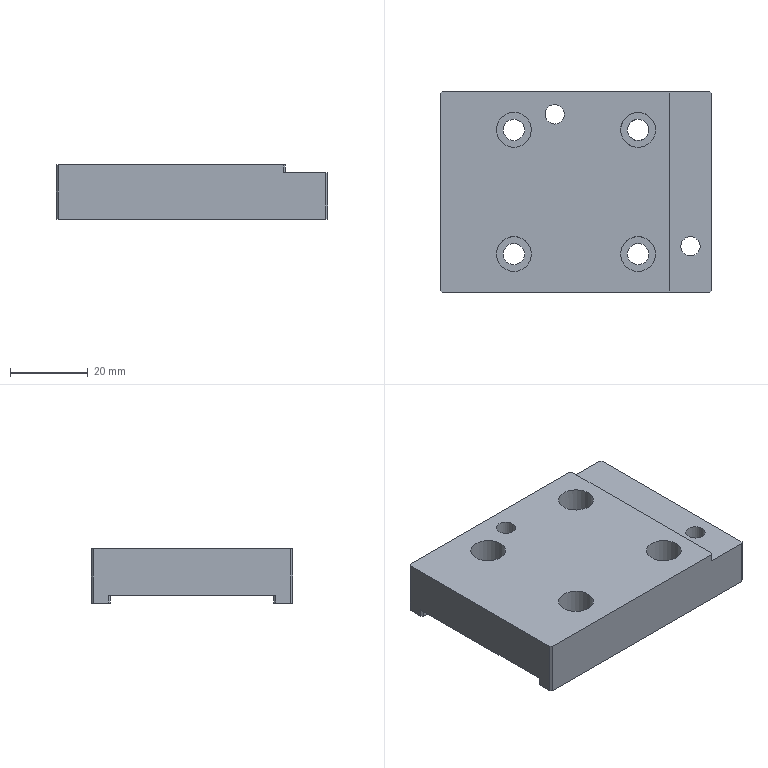CAM job | NX | 3-axis milling, drilling | part box 70 x 52 x 14 mm | stock box 75 x 57 x 20 mm
Tools:
number,name,description,diameter,corner_radius,flute_length,length,flutes
4,D4,平底铣刀-粗,4.0,0.0,25.0,75.0,2
9,D10,平底铣刀-粗,10.0,0.0,35.0,75.0,2
10,D10-J,平底铣刀-精,10.0,0.0,35.0,75.0,2
1,D80R0.8飞刀,圆鼻刀-粗,80.0,0.8,50.0,75.0,2
1,D80R0.8飞刀-J,圆鼻刀-精,80.0,0.8,50.0,75.0,2
2,D6倒角刀,倒角刀,6.0,0.0,3.0,25.0,2
18,M6X1.0,丝锥,5.0,0.0,35.0,50.0,2
15,ZT5,钻头,5.0,0.0,35.0,50.0,2
17,ZT5.5,钻头,5.5,0.0,35.0,50.0,2
Operations:
program,operation,operation_type,tool,method,geometry_group,spindle_rpm,surface_speed,feed_per_tooth,feed_cut,feed_plunge,cut_length_mm,path_length_mm,cut_time_min,machine_time_min
B,面铣自动飞面开粗一刀_1,FaceMilling,D80R0.8飞刀-J,分层开粗-切深K-步距G,W-B,4500.0,1385.0,0.1786,2500.0,100.0,1958.0,3763.618,0.7832,0.9638
B,面铣自动飞面精光一刀_1,FaceMilling,D80R0.8飞刀-J,侧刃精光-切深K-步距G,W-B,4500.0,1385.0,0.0714,1000.0,100.0,178.0,214.0,0.178,0.1816
B,底壁铣分层开粗-中_COPY,VolumeBased25DMillingOperation,D10,分层开粗-切深K-步距G,W-B,8000.0,251.32,0.25,4000.0,100.0,2096.572,2174.132,0.5241,0.5319
B,平面去毛刺6X45L_COPY,SurfaceContour,D6倒角刀,爬面_倒角-切深0-步距G,W-B,6500.0,122.519,0.1154,1500.0,100.0,474.22,1114.357,0.3161,0.3802
B,底壁铣精光底面-中_COPY,VolumeBased25DMillingOperation,D10-J,精光步距切深关,W-B,8000.0,251.32,0.0625,1000.0,100.0,674.853,706.858,0.6749,0.6781
B,底壁铣精光侧面-中-选底面_COPY,VolumeBased25DMillingOperation,D10-J,侧刃精光-切深K-步距G,W-B,8000.0,251.32,0.0625,1000.0,100.0,179.142,251.964,0.1791,0.1864
A,顶面,FaceMilling,D80R0.8飞刀,侧刃精光-切深K-步距G,W-A,4000.0,1005.31,0.125,1000.0,100.0,164.0,200.0,0.164,0.1676
A,外形粗_2,VolumeBased25DMillingOperation,D10,METHOD,W-A,8000.0,251.327,0.3125,5000.0,80.0,5498.974,5551.674,1.1,1.105
A,底壁粗_1,VolumeBased25DMillingOperation,D10,METHOD,W-A,6000.0,113.0,0.2083,3500.0,100.0,516.112,582.815,0.1475,0.1541
A,打点-深0.8,Operation,D6倒角刀,NONE,W-A,8000.0,150.796,0.0312,500.0,90.0,10.8,179.488,0.0216,0.0385
A,通孔-M6螺纹底孔,Operation,ZT5,NONE,W-A,2800.0,43.982,0.0625,350.0,90.0,41.004,173.814,0.1172,0.1304
A,沉头孔-钻孔0段,Operation,ZT5.5,NONE,W-A,2800.0,48.38,0.0179,100.0,90.0,66.609,272.266,0.6661,0.6867
A,铣孔开粗D4_1,CylinderMilling,D4,NONE,W-A,8000.0,100.531,0.075,1200.0,100.0,2398.559,2710.559,1.999,2.03
A,铣孔精光D4_1,CylinderMilling,D4,精光步距切深关,W-A,8000.0,100.531,0.0312,500.0,100.0,192.968,474.968,0.3859,0.4141
A,仅选体,SurfaceContour,D6倒角刀,METHOD,W-A,8000.0,150.796,0.1875,3000.0,100.0,322.033,426.348,0.1073,0.1178
A,铣倒角_1,PlanarMilling,D6倒角刀,METHOD,W-A,8000.0,150.796,0.0312,500.0,100.0,124.848,260.395,0.2497,0.2633
A,铣倒角_2,PlanarMilling,D6倒角刀,NONE,W-A,8000.0,150.796,0.0312,500.0,100.0,148.438,396.876,0.2969,0.3217
A,通孔-攻牙M6,Operation,M6X1.0,METHOD,W-A,500.0,7.854,0.001,1.0,90.0,35.0,159.806,35.0,35.013
A,底精_1,VolumeBased25DMillingOperation,D10-J,METHOD,W-A,6000.0,113.0,0.2083,1200.0,100.0,137.7,180.7,0.1147,0.119
A,底侧精_3,VolumeBased25DMillingOperation,D10-J,METHOD,W-A,6000.0,113.0,0.2083,1200.0,100.0,68.181,111.171,0.0568,0.0611
A,外形半精_2,VolumeBased25DMillingOperation,D10-J,METHOD,W-A,8000.0,251.327,0.0625,1000.0,100.0,279.202,346.603,0.2792,0.2859